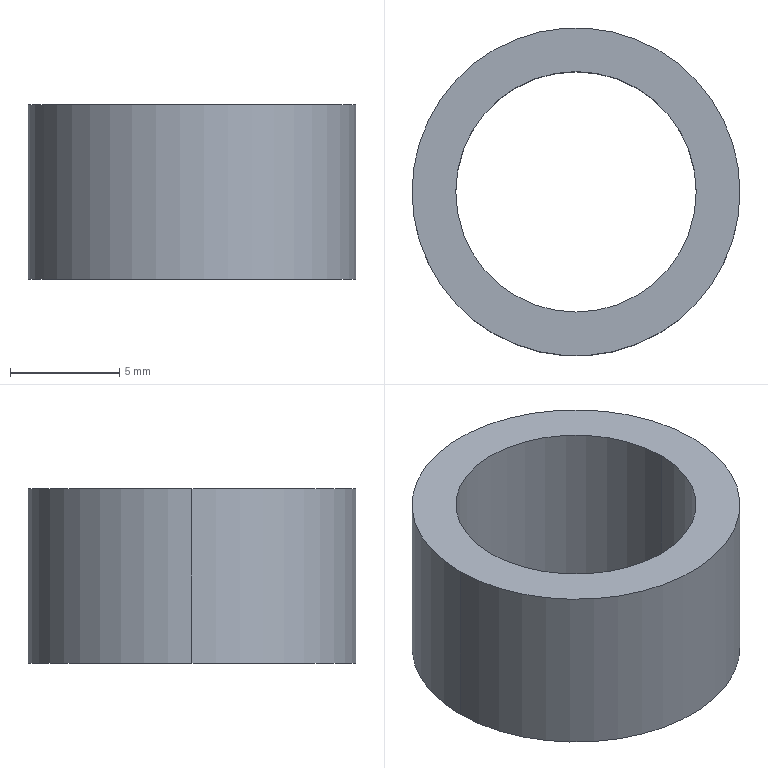Part | SolidWorks | features Extrusion 1 | 1 solid | 6 faces | box 15 x 15 x 8 mm | volume 653.451 mm3 | cylinder 4 | plane 2 | commonest cylinder face diameters 11 x2 15 x2
STEP:
#1=CARTESIAN_POINT('',(-5.5,0.,8.));
#2=VERTEX_POINT('',#1);
#3=CARTESIAN_POINT('',(5.5,0.,8.));
#4=VERTEX_POINT('',#3);
#5=CARTESIAN_POINT('',(0.,0.,8.));
#6=DIRECTION('',(0.,0.,1.));
#7=DIRECTION('',(1.,0.,0.));
#8=AXIS2_PLACEMENT_3D('',#5,#6,#7);
#9=CIRCLE('',#8,5.5);
#10=EDGE_CURVE('',#2,#4,#9,.T.);
#11=ORIENTED_EDGE('',*,*,#10,.T.);
#12=CARTESIAN_POINT('',(5.5,0.,0.));
#13=VERTEX_POINT('',#12);
#14=CARTESIAN_POINT('',(5.5,0.,8.));
#15=DIRECTION('',(0.,0.,-1.));
#16=VECTOR('',#15,1000.);
#17=LINE('',#14,#16);
#18=EDGE_CURVE('',#4,#13,#17,.T.);
#19=ORIENTED_EDGE('',*,*,#18,.T.);
#20=CARTESIAN_POINT('',(-5.5,0.,0.));
#21=VERTEX_POINT('',#20);
#22=CARTESIAN_POINT('',(0.,0.,0.));
#23=DIRECTION('',(0.,0.,1.));
#24=DIRECTION('',(1.,0.,0.));
#25=AXIS2_PLACEMENT_3D('',#22,#23,#24);
#26=CIRCLE('',#25,5.5);
#27=EDGE_CURVE('',#21,#13,#26,.T.);
#28=ORIENTED_EDGE('',*,*,#27,.F.);
#29=CARTESIAN_POINT('',(-5.5,0.,8.));
#30=DIRECTION('',(0.,0.,-1.));
#31=VECTOR('',#30,1000.);
#32=LINE('',#29,#31);
#33=EDGE_CURVE('',#2,#21,#32,.T.);
#34=ORIENTED_EDGE('',*,*,#33,.F.);
#35=EDGE_LOOP('',(#11,#19,#28,#34));
#36=FACE_OUTER_BOUND('',#35,.T.);
#37=CARTESIAN_POINT('',(0.,0.,8.));
#38=DIRECTION('',(0.,0.,-1.));
#39=DIRECTION('',(-1.,0.,0.));
#40=AXIS2_PLACEMENT_3D('',#37,#38,#39);
#41=CYLINDRICAL_SURFACE('',#40,5.5);
#42=ADVANCED_FACE('',(#36),#41,.F.);
#43=CARTESIAN_POINT('',(7.5,0.,8.));
#44=VERTEX_POINT('',#43);
#45=CARTESIAN_POINT('',(-7.5,0.,8.));
#46=VERTEX_POINT('',#45);
#47=CARTESIAN_POINT('',(0.,0.,8.));
#48=DIRECTION('',(0.,0.,1.));
#49=DIRECTION('',(1.,0.,0.));
#50=AXIS2_PLACEMENT_3D('',#47,#48,#49);
#51=CIRCLE('',#50,7.5);
#52=EDGE_CURVE('',#44,#46,#51,.T.);
#53=ORIENTED_EDGE('',*,*,#52,.F.);
#54=CARTESIAN_POINT('',(7.5,0.,0.));
#55=VERTEX_POINT('',#54);
#56=CARTESIAN_POINT('',(7.5,0.,8.));
#57=DIRECTION('',(0.,0.,-1.));
#58=VECTOR('',#57,1000.);
#59=LINE('',#56,#58);
#60=EDGE_CURVE('',#44,#55,#59,.T.);
#61=ORIENTED_EDGE('',*,*,#60,.T.);
#62=CARTESIAN_POINT('',(-7.5,0.,0.));
#63=VERTEX_POINT('',#62);
#64=CARTESIAN_POINT('',(0.,0.,0.));
#65=DIRECTION('',(0.,0.,1.));
#66=DIRECTION('',(1.,0.,0.));
#67=AXIS2_PLACEMENT_3D('',#64,#65,#66);
#68=CIRCLE('',#67,7.5);
#69=EDGE_CURVE('',#55,#63,#68,.T.);
#70=ORIENTED_EDGE('',*,*,#69,.T.);
#71=CARTESIAN_POINT('',(-7.5,0.,8.));
#72=DIRECTION('',(0.,0.,-1.));
#73=VECTOR('',#72,1000.);
#74=LINE('',#71,#73);
#75=EDGE_CURVE('',#46,#63,#74,.T.);
#76=ORIENTED_EDGE('',*,*,#75,.F.);
#77=EDGE_LOOP('',(#53,#61,#70,#76));
#78=FACE_OUTER_BOUND('',#77,.T.);
#79=CARTESIAN_POINT('',(0.,0.,8.));
#80=DIRECTION('',(0.,0.,-1.));
#81=DIRECTION('',(-1.,0.,0.));
#82=AXIS2_PLACEMENT_3D('',#79,#80,#81);
#83=CYLINDRICAL_SURFACE('',#82,7.5);
#84=ADVANCED_FACE('',(#78),#83,.T.);
#85=CARTESIAN_POINT('',(0.,0.,8.));
#86=DIRECTION('',(0.,0.,1.));
#87=DIRECTION('',(1.,0.,0.));
#88=AXIS2_PLACEMENT_3D('',#85,#86,#87);
#89=CIRCLE('',#88,7.5);
#90=EDGE_CURVE('',#46,#44,#89,.T.);
#91=ORIENTED_EDGE('',*,*,#90,.T.);
#92=ORIENTED_EDGE('',*,*,#52,.T.);
#93=EDGE_LOOP('',(#91,#92));
#94=FACE_OUTER_BOUND('',#93,.T.);
#95=ORIENTED_EDGE('',*,*,#10,.F.);
#96=CARTESIAN_POINT('',(0.,0.,8.));
#97=DIRECTION('',(0.,0.,1.));
#98=DIRECTION('',(1.,0.,0.));
#99=AXIS2_PLACEMENT_3D('',#96,#97,#98);
#100=CIRCLE('',#99,5.5);
#101=EDGE_CURVE('',#4,#2,#100,.T.);
#102=ORIENTED_EDGE('',*,*,#101,.F.);
#103=EDGE_LOOP('',(#95,#102));
#104=FACE_BOUND('',#103,.T.);
#105=CARTESIAN_POINT('',(0.,0.,8.));
#106=DIRECTION('',(0.,0.,1.));
#107=DIRECTION('',(1.,0.,0.));
#108=AXIS2_PLACEMENT_3D('',#105,#106,#107);
#109=PLANE('',#108);
#110=ADVANCED_FACE('',(#94,#104),#109,.T.);
#111=CARTESIAN_POINT('',(0.,0.,0.));
#112=DIRECTION('',(0.,0.,1.));
#113=DIRECTION('',(1.,0.,0.));
#114=AXIS2_PLACEMENT_3D('',#111,#112,#113);
#115=CIRCLE('',#114,7.5);
#116=EDGE_CURVE('',#63,#55,#115,.T.);
#117=ORIENTED_EDGE('',*,*,#116,.F.);
#118=ORIENTED_EDGE('',*,*,#69,.F.);
#119=EDGE_LOOP('',(#117,#118));
#120=FACE_OUTER_BOUND('',#119,.T.);
#121=ORIENTED_EDGE('',*,*,#27,.T.);
#122=CARTESIAN_POINT('',(0.,0.,0.));
#123=DIRECTION('',(0.,0.,1.));
#124=DIRECTION('',(1.,0.,0.));
#125=AXIS2_PLACEMENT_3D('',#122,#123,#124);
#126=CIRCLE('',#125,5.5);
#127=EDGE_CURVE('',#13,#21,#126,.T.);
#128=ORIENTED_EDGE('',*,*,#127,.T.);
#129=EDGE_LOOP('',(#121,#128));
#130=FACE_BOUND('',#129,.T.);
#131=CARTESIAN_POINT('',(0.,0.,0.));
#132=DIRECTION('',(0.,0.,1.));
#133=DIRECTION('',(1.,0.,0.));
#134=AXIS2_PLACEMENT_3D('',#131,#132,#133);
#135=PLANE('',#134);
#136=ADVANCED_FACE('',(#120,#130),#135,.F.);
#137=ORIENTED_EDGE('',*,*,#60,.F.);
#138=ORIENTED_EDGE('',*,*,#90,.F.);
#139=ORIENTED_EDGE('',*,*,#75,.T.);
#140=ORIENTED_EDGE('',*,*,#116,.T.);
#141=EDGE_LOOP('',(#137,#138,#139,#140));
#142=FACE_OUTER_BOUND('',#141,.T.);
#143=CARTESIAN_POINT('',(0.,0.,8.));
#144=DIRECTION('',(0.,0.,-1.));
#145=DIRECTION('',(-1.,0.,0.));
#146=AXIS2_PLACEMENT_3D('',#143,#144,#145);
#147=CYLINDRICAL_SURFACE('',#146,7.5);
#148=ADVANCED_FACE('',(#142),#147,.T.);
#149=ORIENTED_EDGE('',*,*,#18,.F.);
#150=ORIENTED_EDGE('',*,*,#101,.T.);
#151=ORIENTED_EDGE('',*,*,#33,.T.);
#152=ORIENTED_EDGE('',*,*,#127,.F.);
#153=EDGE_LOOP('',(#149,#150,#151,#152));
#154=FACE_OUTER_BOUND('',#153,.T.);
#155=CARTESIAN_POINT('',(0.,0.,8.));
#156=DIRECTION('',(0.,0.,-1.));
#157=DIRECTION('',(-1.,0.,0.));
#158=AXIS2_PLACEMENT_3D('',#155,#156,#157);
#159=CYLINDRICAL_SURFACE('',#158,5.5);
#160=ADVANCED_FACE('',(#154),#159,.F.);
#161=CLOSED_SHELL('',(#42,#84,#110,#136,#148,#160));
#162=MANIFOLD_SOLID_BREP('',#161);
#163=CARTESIAN_POINT('',(0.,0.,0.));
#164=DIRECTION('',(0.,0.,1.));
#165=DIRECTION('',(1.,0.,0.));
#166=AXIS2_PLACEMENT_3D('',#163,#164,#165);
#167=(LENGTH_UNIT()NAMED_UNIT(*)SI_UNIT(.MILLI.,.METRE.));
#168=UNCERTAINTY_MEASURE_WITH_UNIT(LENGTH_MEASURE(0.00001),#167,'','');
#169=(NAMED_UNIT(*)PLANE_ANGLE_UNIT()SI_UNIT($,.RADIAN.));
#170=(NAMED_UNIT(*)SI_UNIT($,.STERADIAN.)SOLID_ANGLE_UNIT());
#171=(GEOMETRIC_REPRESENTATION_CONTEXT(3)GLOBAL_UNCERTAINTY_ASSIGNED_CONTEXT((#168))GLOBAL_UNIT_ASSIGNED_CONTEXT((#167,#169,#170))REPRESENTATION_CONTEXT('',''));
#172=ADVANCED_BREP_SHAPE_REPRESENTATION('',(#162,#166),#171);